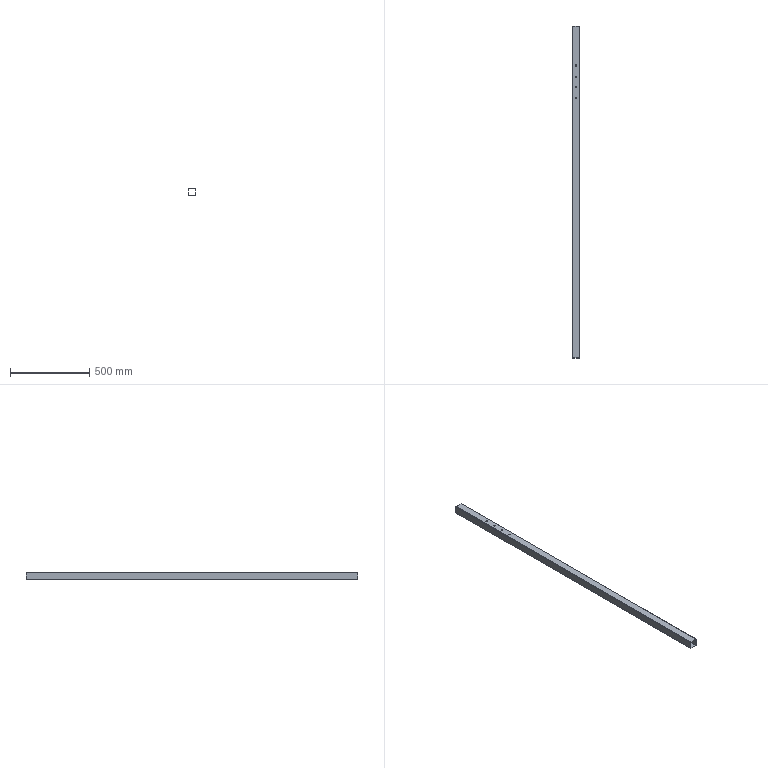Part | SolidWorks | features Extrusion 1, ICE 1 | 1 solid | 34 faces | box 50 x 2097 x 50 mm | volume 900278 mm3 | cylinder 24 | plane 10 | commonest cylinder face diameters 8 x16 2.3 x4 6.9 x4
STEP:
#1=CARTESIAN_POINT('',(4.,1847.,25.));
#2=VERTEX_POINT('',#1);
#3=CARTESIAN_POINT('',(-4.,1847.,25.));
#4=VERTEX_POINT('',#3);
#5=CARTESIAN_POINT('',(0.,1847.,25.));
#6=DIRECTION('',(0.,0.,-1.));
#7=DIRECTION('',(-1.,0.,0.));
#8=AXIS2_PLACEMENT_3D('',#5,#6,#7);
#9=CIRCLE('',#8,4.);
#10=EDGE_CURVE('',#2,#4,#9,.T.);
#11=ORIENTED_EDGE('',*,*,#10,.F.);
#12=CARTESIAN_POINT('',(4.,1847.,22.7));
#13=VERTEX_POINT('',#12);
#14=CARTESIAN_POINT('',(4.,1847.,25.));
#15=DIRECTION('',(0.,0.,-1.));
#16=VECTOR('',#15,1000.);
#17=LINE('',#14,#16);
#18=EDGE_CURVE('',#2,#13,#17,.T.);
#19=ORIENTED_EDGE('',*,*,#18,.T.);
#20=CARTESIAN_POINT('',(-4.,1847.,22.7));
#21=VERTEX_POINT('',#20);
#22=CARTESIAN_POINT('',(0.,1847.,22.7));
#23=DIRECTION('',(0.,0.,-1.));
#24=DIRECTION('',(-1.,0.,0.));
#25=AXIS2_PLACEMENT_3D('',#22,#23,#24);
#26=CIRCLE('',#25,4.);
#27=EDGE_CURVE('',#13,#21,#26,.T.);
#28=ORIENTED_EDGE('',*,*,#27,.T.);
#29=CARTESIAN_POINT('',(-4.,1847.,25.));
#30=DIRECTION('',(0.,0.,-1.));
#31=VECTOR('',#30,1000.);
#32=LINE('',#29,#31);
#33=EDGE_CURVE('',#4,#21,#32,.T.);
#34=ORIENTED_EDGE('',*,*,#33,.F.);
#35=EDGE_LOOP('',(#11,#19,#28,#34));
#36=FACE_OUTER_BOUND('',#35,.T.);
#37=CARTESIAN_POINT('',(0.,1847.,25.));
#38=DIRECTION('',(0.,0.,-1.));
#39=DIRECTION('',(-1.,0.,0.));
#40=AXIS2_PLACEMENT_3D('',#37,#38,#39);
#41=CYLINDRICAL_SURFACE('',#40,4.);
#42=ADVANCED_FACE('',(#36),#41,.F.);
#43=CARTESIAN_POINT('',(4.,1777.,25.));
#44=VERTEX_POINT('',#43);
#45=CARTESIAN_POINT('',(-4.,1777.,25.));
#46=VERTEX_POINT('',#45);
#47=CARTESIAN_POINT('',(0.,1777.,25.));
#48=DIRECTION('',(0.,0.,-1.));
#49=DIRECTION('',(-1.,0.,0.));
#50=AXIS2_PLACEMENT_3D('',#47,#48,#49);
#51=CIRCLE('',#50,4.);
#52=EDGE_CURVE('',#44,#46,#51,.T.);
#53=ORIENTED_EDGE('',*,*,#52,.F.);
#54=CARTESIAN_POINT('',(4.,1777.,22.7));
#55=VERTEX_POINT('',#54);
#56=CARTESIAN_POINT('',(4.,1777.,25.));
#57=DIRECTION('',(0.,0.,-1.));
#58=VECTOR('',#57,1000.);
#59=LINE('',#56,#58);
#60=EDGE_CURVE('',#44,#55,#59,.T.);
#61=ORIENTED_EDGE('',*,*,#60,.T.);
#62=CARTESIAN_POINT('',(-4.,1777.,22.7));
#63=VERTEX_POINT('',#62);
#64=CARTESIAN_POINT('',(0.,1777.,22.7));
#65=DIRECTION('',(0.,0.,-1.));
#66=DIRECTION('',(-1.,0.,0.));
#67=AXIS2_PLACEMENT_3D('',#64,#65,#66);
#68=CIRCLE('',#67,4.);
#69=EDGE_CURVE('',#55,#63,#68,.T.);
#70=ORIENTED_EDGE('',*,*,#69,.T.);
#71=CARTESIAN_POINT('',(-4.,1777.,25.));
#72=DIRECTION('',(0.,0.,-1.));
#73=VECTOR('',#72,1000.);
#74=LINE('',#71,#73);
#75=EDGE_CURVE('',#46,#63,#74,.T.);
#76=ORIENTED_EDGE('',*,*,#75,.F.);
#77=EDGE_LOOP('',(#53,#61,#70,#76));
#78=FACE_OUTER_BOUND('',#77,.T.);
#79=CARTESIAN_POINT('',(0.,1777.,25.));
#80=DIRECTION('',(0.,0.,-1.));
#81=DIRECTION('',(-1.,0.,0.));
#82=AXIS2_PLACEMENT_3D('',#79,#80,#81);
#83=CYLINDRICAL_SURFACE('',#82,4.);
#84=ADVANCED_FACE('',(#78),#83,.F.);
#85=CARTESIAN_POINT('',(4.,1712.,25.));
#86=VERTEX_POINT('',#85);
#87=CARTESIAN_POINT('',(-4.,1712.,25.));
#88=VERTEX_POINT('',#87);
#89=CARTESIAN_POINT('',(0.,1712.,25.));
#90=DIRECTION('',(0.,0.,-1.));
#91=DIRECTION('',(-1.,0.,0.));
#92=AXIS2_PLACEMENT_3D('',#89,#90,#91);
#93=CIRCLE('',#92,4.);
#94=EDGE_CURVE('',#86,#88,#93,.T.);
#95=ORIENTED_EDGE('',*,*,#94,.F.);
#96=CARTESIAN_POINT('',(4.,1712.,22.7));
#97=VERTEX_POINT('',#96);
#98=CARTESIAN_POINT('',(4.,1712.,25.));
#99=DIRECTION('',(0.,0.,-1.));
#100=VECTOR('',#99,1000.);
#101=LINE('',#98,#100);
#102=EDGE_CURVE('',#86,#97,#101,.T.);
#103=ORIENTED_EDGE('',*,*,#102,.T.);
#104=CARTESIAN_POINT('',(-4.,1712.,22.7));
#105=VERTEX_POINT('',#104);
#106=CARTESIAN_POINT('',(0.,1712.,22.7));
#107=DIRECTION('',(0.,0.,-1.));
#108=DIRECTION('',(-1.,0.,0.));
#109=AXIS2_PLACEMENT_3D('',#106,#107,#108);
#110=CIRCLE('',#109,4.);
#111=EDGE_CURVE('',#97,#105,#110,.T.);
#112=ORIENTED_EDGE('',*,*,#111,.T.);
#113=CARTESIAN_POINT('',(-4.,1712.,25.));
#114=DIRECTION('',(0.,0.,-1.));
#115=VECTOR('',#114,1000.);
#116=LINE('',#113,#115);
#117=EDGE_CURVE('',#88,#105,#116,.T.);
#118=ORIENTED_EDGE('',*,*,#117,.F.);
#119=EDGE_LOOP('',(#95,#103,#112,#118));
#120=FACE_OUTER_BOUND('',#119,.T.);
#121=CARTESIAN_POINT('',(0.,1712.,25.));
#122=DIRECTION('',(0.,0.,-1.));
#123=DIRECTION('',(-1.,0.,0.));
#124=AXIS2_PLACEMENT_3D('',#121,#122,#123);
#125=CYLINDRICAL_SURFACE('',#124,4.);
#126=ADVANCED_FACE('',(#120),#125,.F.);
#127=CARTESIAN_POINT('',(4.,1642.,25.));
#128=VERTEX_POINT('',#127);
#129=CARTESIAN_POINT('',(-4.,1642.,25.));
#130=VERTEX_POINT('',#129);
#131=CARTESIAN_POINT('',(0.,1642.,25.));
#132=DIRECTION('',(0.,0.,-1.));
#133=DIRECTION('',(-1.,0.,0.));
#134=AXIS2_PLACEMENT_3D('',#131,#132,#133);
#135=CIRCLE('',#134,4.);
#136=EDGE_CURVE('',#128,#130,#135,.T.);
#137=ORIENTED_EDGE('',*,*,#136,.F.);
#138=CARTESIAN_POINT('',(4.,1642.,22.7));
#139=VERTEX_POINT('',#138);
#140=CARTESIAN_POINT('',(4.,1642.,25.));
#141=DIRECTION('',(0.,0.,-1.));
#142=VECTOR('',#141,1000.);
#143=LINE('',#140,#142);
#144=EDGE_CURVE('',#128,#139,#143,.T.);
#145=ORIENTED_EDGE('',*,*,#144,.T.);
#146=CARTESIAN_POINT('',(-4.,1642.,22.7));
#147=VERTEX_POINT('',#146);
#148=CARTESIAN_POINT('',(0.,1642.,22.7));
#149=DIRECTION('',(0.,0.,-1.));
#150=DIRECTION('',(-1.,0.,0.));
#151=AXIS2_PLACEMENT_3D('',#148,#149,#150);
#152=CIRCLE('',#151,4.);
#153=EDGE_CURVE('',#139,#147,#152,.T.);
#154=ORIENTED_EDGE('',*,*,#153,.T.);
#155=CARTESIAN_POINT('',(-4.,1642.,25.));
#156=DIRECTION('',(0.,0.,-1.));
#157=VECTOR('',#156,1000.);
#158=LINE('',#155,#157);
#159=EDGE_CURVE('',#130,#147,#158,.T.);
#160=ORIENTED_EDGE('',*,*,#159,.F.);
#161=EDGE_LOOP('',(#137,#145,#154,#160));
#162=FACE_OUTER_BOUND('',#161,.T.);
#163=CARTESIAN_POINT('',(0.,1642.,25.));
#164=DIRECTION('',(0.,0.,-1.));
#165=DIRECTION('',(-1.,0.,0.));
#166=AXIS2_PLACEMENT_3D('',#163,#164,#165);
#167=CYLINDRICAL_SURFACE('',#166,4.);
#168=ADVANCED_FACE('',(#162),#167,.F.);
#169=CARTESIAN_POINT('',(-4.,1847.,-22.7));
#170=VERTEX_POINT('',#169);
#171=CARTESIAN_POINT('',(4.,1847.,-22.7));
#172=VERTEX_POINT('',#171);
#173=CARTESIAN_POINT('',(0.,1847.,-22.7));
#174=DIRECTION('',(0.,0.,1.));
#175=DIRECTION('',(1.,0.,0.));
#176=AXIS2_PLACEMENT_3D('',#173,#174,#175);
#177=CIRCLE('',#176,4.);
#178=EDGE_CURVE('',#170,#172,#177,.T.);
#179=ORIENTED_EDGE('',*,*,#178,.T.);
#180=CARTESIAN_POINT('',(4.,1847.,-25.));
#181=VERTEX_POINT('',#180);
#182=CARTESIAN_POINT('',(4.,1847.,25.));
#183=DIRECTION('',(0.,0.,-1.));
#184=VECTOR('',#183,1000.);
#185=LINE('',#182,#184);
#186=EDGE_CURVE('',#172,#181,#185,.T.);
#187=ORIENTED_EDGE('',*,*,#186,.T.);
#188=CARTESIAN_POINT('',(-4.,1847.,-25.));
#189=VERTEX_POINT('',#188);
#190=CARTESIAN_POINT('',(0.,1847.,-25.));
#191=DIRECTION('',(0.,0.,1.));
#192=DIRECTION('',(1.,0.,0.));
#193=AXIS2_PLACEMENT_3D('',#190,#191,#192);
#194=CIRCLE('',#193,4.);
#195=EDGE_CURVE('',#189,#181,#194,.T.);
#196=ORIENTED_EDGE('',*,*,#195,.F.);
#197=CARTESIAN_POINT('',(-4.,1847.,25.));
#198=DIRECTION('',(0.,0.,-1.));
#199=VECTOR('',#198,1000.);
#200=LINE('',#197,#199);
#201=EDGE_CURVE('',#170,#189,#200,.T.);
#202=ORIENTED_EDGE('',*,*,#201,.F.);
#203=EDGE_LOOP('',(#179,#187,#196,#202));
#204=FACE_OUTER_BOUND('',#203,.T.);
#205=CARTESIAN_POINT('',(0.,1847.,25.));
#206=DIRECTION('',(0.,0.,-1.));
#207=DIRECTION('',(-1.,0.,0.));
#208=AXIS2_PLACEMENT_3D('',#205,#206,#207);
#209=CYLINDRICAL_SURFACE('',#208,4.);
#210=ADVANCED_FACE('',(#204),#209,.F.);
#211=CARTESIAN_POINT('',(-4.,1777.,-22.7));
#212=VERTEX_POINT('',#211);
#213=CARTESIAN_POINT('',(4.,1777.,-22.7));
#214=VERTEX_POINT('',#213);
#215=CARTESIAN_POINT('',(0.,1777.,-22.7));
#216=DIRECTION('',(0.,0.,1.));
#217=DIRECTION('',(1.,0.,0.));
#218=AXIS2_PLACEMENT_3D('',#215,#216,#217);
#219=CIRCLE('',#218,4.);
#220=EDGE_CURVE('',#212,#214,#219,.T.);
#221=ORIENTED_EDGE('',*,*,#220,.T.);
#222=CARTESIAN_POINT('',(4.,1777.,-25.));
#223=VERTEX_POINT('',#222);
#224=CARTESIAN_POINT('',(4.,1777.,25.));
#225=DIRECTION('',(0.,0.,-1.));
#226=VECTOR('',#225,1000.);
#227=LINE('',#224,#226);
#228=EDGE_CURVE('',#214,#223,#227,.T.);
#229=ORIENTED_EDGE('',*,*,#228,.T.);
#230=CARTESIAN_POINT('',(-4.,1777.,-25.));
#231=VERTEX_POINT('',#230);
#232=CARTESIAN_POINT('',(0.,1777.,-25.));
#233=DIRECTION('',(0.,0.,1.));
#234=DIRECTION('',(1.,0.,0.));
#235=AXIS2_PLACEMENT_3D('',#232,#233,#234);
#236=CIRCLE('',#235,4.);
#237=EDGE_CURVE('',#231,#223,#236,.T.);
#238=ORIENTED_EDGE('',*,*,#237,.F.);
#239=CARTESIAN_POINT('',(-4.,1777.,25.));
#240=DIRECTION('',(0.,0.,-1.));
#241=VECTOR('',#240,1000.);
#242=LINE('',#239,#241);
#243=EDGE_CURVE('',#212,#231,#242,.T.);
#244=ORIENTED_EDGE('',*,*,#243,.F.);
#245=EDGE_LOOP('',(#221,#229,#238,#244));
#246=FACE_OUTER_BOUND('',#245,.T.);
#247=CARTESIAN_POINT('',(0.,1777.,25.));
#248=DIRECTION('',(0.,0.,-1.));
#249=DIRECTION('',(-1.,0.,0.));
#250=AXIS2_PLACEMENT_3D('',#247,#248,#249);
#251=CYLINDRICAL_SURFACE('',#250,4.);
#252=ADVANCED_FACE('',(#246),#251,.F.);
#253=CARTESIAN_POINT('',(-4.,1712.,-22.7));
#254=VERTEX_POINT('',#253);
#255=CARTESIAN_POINT('',(4.,1712.,-22.7));
#256=VERTEX_POINT('',#255);
#257=CARTESIAN_POINT('',(0.,1712.,-22.7));
#258=DIRECTION('',(0.,0.,1.));
#259=DIRECTION('',(1.,0.,0.));
#260=AXIS2_PLACEMENT_3D('',#257,#258,#259);
#261=CIRCLE('',#260,4.);
#262=EDGE_CURVE('',#254,#256,#261,.T.);
#263=ORIENTED_EDGE('',*,*,#262,.T.);
#264=CARTESIAN_POINT('',(4.,1712.,-25.));
#265=VERTEX_POINT('',#264);
#266=CARTESIAN_POINT('',(4.,1712.,25.));
#267=DIRECTION('',(0.,0.,-1.));
#268=VECTOR('',#267,1000.);
#269=LINE('',#266,#268);
#270=EDGE_CURVE('',#256,#265,#269,.T.);
#271=ORIENTED_EDGE('',*,*,#270,.T.);
#272=CARTESIAN_POINT('',(-4.,1712.,-25.));
#273=VERTEX_POINT('',#272);
#274=CARTESIAN_POINT('',(0.,1712.,-25.));
#275=DIRECTION('',(0.,0.,1.));
#276=DIRECTION('',(1.,0.,0.));
#277=AXIS2_PLACEMENT_3D('',#274,#275,#276);
#278=CIRCLE('',#277,4.);
#279=EDGE_CURVE('',#273,#265,#278,.T.);
#280=ORIENTED_EDGE('',*,*,#279,.F.);
#281=CARTESIAN_POINT('',(-4.,1712.,25.));
#282=DIRECTION('',(0.,0.,-1.));
#283=VECTOR('',#282,1000.);
#284=LINE('',#281,#283);
#285=EDGE_CURVE('',#254,#273,#284,.T.);
#286=ORIENTED_EDGE('',*,*,#285,.F.);
#287=EDGE_LOOP('',(#263,#271,#280,#286));
#288=FACE_OUTER_BOUND('',#287,.T.);
#289=CARTESIAN_POINT('',(0.,1712.,25.));
#290=DIRECTION('',(0.,0.,-1.));
#291=DIRECTION('',(-1.,0.,0.));
#292=AXIS2_PLACEMENT_3D('',#289,#290,#291);
#293=CYLINDRICAL_SURFACE('',#292,4.);
#294=ADVANCED_FACE('',(#288),#293,.F.);
#295=CARTESIAN_POINT('',(-4.,1642.,-22.7));
#296=VERTEX_POINT('',#295);
#297=CARTESIAN_POINT('',(4.,1642.,-22.7));
#298=VERTEX_POINT('',#297);
#299=CARTESIAN_POINT('',(0.,1642.,-22.7));
#300=DIRECTION('',(0.,0.,1.));
#301=DIRECTION('',(1.,0.,0.));
#302=AXIS2_PLACEMENT_3D('',#299,#300,#301);
#303=CIRCLE('',#302,4.);
#304=EDGE_CURVE('',#296,#298,#303,.T.);
#305=ORIENTED_EDGE('',*,*,#304,.T.);
#306=CARTESIAN_POINT('',(4.,1642.,-25.));
#307=VERTEX_POINT('',#306);
#308=CARTESIAN_POINT('',(4.,1642.,25.));
#309=DIRECTION('',(0.,0.,-1.));
#310=VECTOR('',#309,1000.);
#311=LINE('',#308,#310);
#312=EDGE_CURVE('',#298,#307,#311,.T.);
#313=ORIENTED_EDGE('',*,*,#312,.T.);
#314=CARTESIAN_POINT('',(-4.,1642.,-25.));
#315=VERTEX_POINT('',#314);
#316=CARTESIAN_POINT('',(0.,1642.,-25.));
#317=DIRECTION('',(0.,0.,1.));
#318=DIRECTION('',(1.,0.,0.));
#319=AXIS2_PLACEMENT_3D('',#316,#317,#318);
#320=CIRCLE('',#319,4.);
#321=EDGE_CURVE('',#315,#307,#320,.T.);
#322=ORIENTED_EDGE('',*,*,#321,.F.);
#323=CARTESIAN_POINT('',(-4.,1642.,25.));
#324=DIRECTION('',(0.,0.,-1.));
#325=VECTOR('',#324,1000.);
#326=LINE('',#323,#325);
#327=EDGE_CURVE('',#296,#315,#326,.T.);
#328=ORIENTED_EDGE('',*,*,#327,.F.);
#329=EDGE_LOOP('',(#305,#313,#322,#328));
#330=FACE_OUTER_BOUND('',#329,.T.);
#331=CARTESIAN_POINT('',(0.,1642.,25.));
#332=DIRECTION('',(0.,0.,-1.));
#333=DIRECTION('',(-1.,0.,0.));
#334=AXIS2_PLACEMENT_3D('',#331,#332,#333);
#335=CYLINDRICAL_SURFACE('',#334,4.);
#336=ADVANCED_FACE('',(#330),#335,.F.);
#337=CARTESIAN_POINT('',(25.,2097.,-21.55));
#338=VERTEX_POINT('',#337);
#339=CARTESIAN_POINT('',(21.55,2097.,-25.));
#340=VERTEX_POINT('',#339);
#341=CARTESIAN_POINT('',(21.55,2097.,-21.55));
#342=DIRECTION('',(0.,1.,0.));
#343=DIRECTION('',(0.,0.,-1.));
#344=AXIS2_PLACEMENT_3D('',#341,#342,#343);
#345=CIRCLE('',#344,3.45);
#346=EDGE_CURVE('',#338,#340,#345,.T.);
#347=ORIENTED_EDGE('',*,*,#346,.T.);
#348=CARTESIAN_POINT('',(-21.55,2097.,-25.));
#349=VERTEX_POINT('',#348);
#350=CARTESIAN_POINT('',(-21.55,2097.,-25.));
#351=DIRECTION('',(-1.,0.,0.));
#352=VECTOR('',#351,1000.);
#353=LINE('',#350,#352);
#354=EDGE_CURVE('',#340,#349,#353,.T.);
#355=ORIENTED_EDGE('',*,*,#354,.T.);
#356=CARTESIAN_POINT('',(-25.,2097.,-21.55));
#357=VERTEX_POINT('',#356);
#358=CARTESIAN_POINT('',(-21.55,2097.,-21.55));
#359=DIRECTION('',(0.,1.,0.));
#360=DIRECTION('',(0.,0.,-1.));
#361=AXIS2_PLACEMENT_3D('',#358,#359,#360);
#362=CIRCLE('',#361,3.45);
#363=EDGE_CURVE('',#349,#357,#362,.T.);
#364=ORIENTED_EDGE('',*,*,#363,.T.);
#365=CARTESIAN_POINT('',(-25.,2097.,21.55));
#366=VERTEX_POINT('',#365);
#367=CARTESIAN_POINT('',(-25.,2097.,21.55));
#368=DIRECTION('',(0.,0.,1.));
#369=VECTOR('',#368,1000.);
#370=LINE('',#367,#369);
#371=EDGE_CURVE('',#357,#366,#370,.T.);
#372=ORIENTED_EDGE('',*,*,#371,.T.);
#373=CARTESIAN_POINT('',(-21.55,2097.,25.));
#374=VERTEX_POINT('',#373);
#375=CARTESIAN_POINT('',(-21.55,2097.,21.55));
#376=DIRECTION('',(0.,1.,0.));
#377=DIRECTION('',(0.,0.,-1.));
#378=AXIS2_PLACEMENT_3D('',#375,#376,#377);
#379=CIRCLE('',#378,3.45);
#380=EDGE_CURVE('',#366,#374,#379,.T.);
#381=ORIENTED_EDGE('',*,*,#380,.T.);
#382=CARTESIAN_POINT('',(21.55,2097.,25.));
#383=VERTEX_POINT('',#382);
#384=CARTESIAN_POINT('',(-21.55,2097.,25.));
#385=DIRECTION('',(1.,0.,0.));
#386=VECTOR('',#385,1000.);
#387=LINE('',#384,#386);
#388=EDGE_CURVE('',#374,#383,#387,.T.);
#389=ORIENTED_EDGE('',*,*,#388,.T.);
#390=CARTESIAN_POINT('',(25.,2097.,21.55));
#391=VERTEX_POINT('',#390);
#392=CARTESIAN_POINT('',(21.55,2097.,21.55));
#393=DIRECTION('',(0.,1.,0.));
#394=DIRECTION('',(0.,0.,1.));
#395=AXIS2_PLACEMENT_3D('',#392,#393,#394);
#396=CIRCLE('',#395,3.45);
#397=EDGE_CURVE('',#383,#391,#396,.T.);
#398=ORIENTED_EDGE('',*,*,#397,.T.);
#399=CARTESIAN_POINT('',(25.,2097.,21.55));
#400=DIRECTION('',(0.,0.,-1.));
#401=VECTOR('',#400,1000.);
#402=LINE('',#399,#401);
#403=EDGE_CURVE('',#391,#338,#402,.T.);
#404=ORIENTED_EDGE('',*,*,#403,.T.);
#405=EDGE_LOOP('',(#347,#355,#364,#372,#381,#389,#398,#404));
#406=FACE_OUTER_BOUND('',#405,.T.);
#407=CARTESIAN_POINT('',(-22.7,2097.,21.55));
#408=VERTEX_POINT('',#407);
#409=CARTESIAN_POINT('',(-21.55,2097.,22.7));
#410=VERTEX_POINT('',#409);
#411=CARTESIAN_POINT('',(-21.55,2097.,21.55));
#412=DIRECTION('',(0.,1.,0.));
#413=DIRECTION('',(0.,0.,-1.));
#414=AXIS2_PLACEMENT_3D('',#411,#412,#413);
#415=CIRCLE('',#414,1.15);
#416=EDGE_CURVE('',#408,#410,#415,.T.);
#417=ORIENTED_EDGE('',*,*,#416,.F.);
#418=CARTESIAN_POINT('',(-22.7,2097.,-21.55));
#419=VERTEX_POINT('',#418);
#420=CARTESIAN_POINT('',(-22.7,2097.,21.55));
#421=DIRECTION('',(0.,0.,1.));
#422=VECTOR('',#421,1000.);
#423=LINE('',#420,#422);
#424=EDGE_CURVE('',#419,#408,#423,.T.);
#425=ORIENTED_EDGE('',*,*,#424,.F.);
#426=CARTESIAN_POINT('',(-21.55,2097.,-22.7));
#427=VERTEX_POINT('',#426);
#428=CARTESIAN_POINT('',(-21.55,2097.,-21.55));
#429=DIRECTION('',(0.,1.,0.));
#430=DIRECTION('',(0.,0.,-1.));
#431=AXIS2_PLACEMENT_3D('',#428,#429,#430);
#432=CIRCLE('',#431,1.15);
#433=EDGE_CURVE('',#427,#419,#432,.T.);
#434=ORIENTED_EDGE('',*,*,#433,.F.);
#435=CARTESIAN_POINT('',(21.55,2097.,-22.7));
#436=VERTEX_POINT('',#435);
#437=CARTESIAN_POINT('',(-21.55,2097.,-22.7));
#438=DIRECTION('',(-1.,0.,0.));
#439=VECTOR('',#438,1000.);
#440=LINE('',#437,#439);
#441=EDGE_CURVE('',#436,#427,#440,.T.);
#442=ORIENTED_EDGE('',*,*,#441,.F.);
#443=CARTESIAN_POINT('',(22.7,2097.,-21.55));
#444=VERTEX_POINT('',#443);
#445=CARTESIAN_POINT('',(21.55,2097.,-21.55));
#446=DIRECTION('',(0.,1.,0.));
#447=DIRECTION('',(0.,0.,-1.));
#448=AXIS2_PLACEMENT_3D('',#445,#446,#447);
#449=CIRCLE('',#448,1.15);
#450=EDGE_CURVE('',#444,#436,#449,.T.);
#451=ORIENTED_EDGE('',*,*,#450,.F.);
#452=CARTESIAN_POINT('',(22.7,2097.,21.55));
#453=VERTEX_POINT('',#452);
#454=CARTESIAN_POINT('',(22.7,2097.,21.55));
#455=DIRECTION('',(0.,0.,-1.));
#456=VECTOR('',#455,1000.);
#457=LINE('',#454,#456);
#458=EDGE_CURVE('',#453,#444,#457,.T.);
#459=ORIENTED_EDGE('',*,*,#458,.F.);
#460=CARTESIAN_POINT('',(21.55,2097.,22.7));
#461=VERTEX_POINT('',#460);
#462=CARTESIAN_POINT('',(21.55,2097.,21.55));
#463=DIRECTION('',(0.,1.,0.));
#464=DIRECTION('',(0.,0.,1.));
#465=AXIS2_PLACEMENT_3D('',#462,#463,#464);
#466=CIRCLE('',#465,1.15);
#467=EDGE_CURVE('',#461,#453,#466,.T.);
#468=ORIENTED_EDGE('',*,*,#467,.F.);
#469=CARTESIAN_POINT('',(-21.55,2097.,22.7));
#470=DIRECTION('',(1.,0.,0.));
#471=VECTOR('',#470,1000.);
#472=LINE('',#469,#471);
#473=EDGE_CURVE('',#410,#461,#472,.T.);
#474=ORIENTED_EDGE('',*,*,#473,.F.);
#475=EDGE_LOOP('',(#417,#425,#434,#442,#451,#459,#468,#474));
#476=FACE_BOUND('',#475,.T.);
#477=CARTESIAN_POINT('',(21.55,2097.,-21.55));
#478=DIRECTION('',(0.,-1.,0.));
#479=DIRECTION('',(0.,0.,-1.));
#480=AXIS2_PLACEMENT_3D('',#477,#478,#479);
#481=PLANE('',#480);
#482=ADVANCED_FACE('',(#406,#476),#481,.F.);
#483=CARTESIAN_POINT('',(25.,0.,-21.55));
#484=VERTEX_POINT('',#483);
#485=CARTESIAN_POINT('',(21.55,0.,-25.));
#486=VERTEX_POINT('',#485);
#487=CARTESIAN_POINT('',(21.55,0.,-21.55));
#488=DIRECTION('',(0.,1.,0.));
#489=DIRECTION('',(0.,0.,-1.));
#490=AXIS2_PLACEMENT_3D('',#487,#488,#489);
#491=CIRCLE('',#490,3.45);
#492=EDGE_CURVE('',#484,#486,#491,.T.);
#493=ORIENTED_EDGE('',*,*,#492,.F.);
#494=CARTESIAN_POINT('',(25.,0.,21.55));
#495=VERTEX_POINT('',#494);
#496=CARTESIAN_POINT('',(25.,0.,21.55));
#497=DIRECTION('',(0.,0.,-1.));
#498=VECTOR('',#497,1000.);
#499=LINE('',#496,#498);
#500=EDGE_CURVE('',#495,#484,#499,.T.);
#501=ORIENTED_EDGE('',*,*,#500,.F.);
#502=CARTESIAN_POINT('',(21.55,0.,25.));
#503=VERTEX_POINT('',#502);
#504=CARTESIAN_POINT('',(21.55,0.,21.55));
#505=DIRECTION('',(0.,1.,0.));
#506=DIRECTION('',(0.,0.,1.));
#507=AXIS2_PLACEMENT_3D('',#504,#505,#506);
#508=CIRCLE('',#507,3.45);
#509=EDGE_CURVE('',#503,#495,#508,.T.);
#510=ORIENTED_EDGE('',*,*,#509,.F.);
#511=CARTESIAN_POINT('',(-21.55,0.,25.));
#512=VERTEX_POINT('',#511);
#513=CARTESIAN_POINT('',(-21.55,0.,25.));
#514=DIRECTION('',(1.,0.,0.));
#515=VECTOR('',#514,1000.);
#516=LINE('',#513,#515);
#517=EDGE_CURVE('',#512,#503,#516,.T.);
#518=ORIENTED_EDGE('',*,*,#517,.F.);
#519=CARTESIAN_POINT('',(-25.,0.,21.55));
#520=VERTEX_POINT('',#519);
#521=CARTESIAN_POINT('',(-21.55,0.,21.55));
#522=DIRECTION('',(0.,1.,0.));
#523=DIRECTION('',(0.,0.,-1.));
#524=AXIS2_PLACEMENT_3D('',#521,#522,#523);
#525=CIRCLE('',#524,3.45);
#526=EDGE_CURVE('',#520,#512,#525,.T.);
#527=ORIENTED_EDGE('',*,*,#526,.F.);
#528=CARTESIAN_POINT('',(-25.,0.,-21.55));
#529=VERTEX_POINT('',#528);
#530=CARTESIAN_POINT('',(-25.,0.,21.55));
#531=DIRECTION('',(0.,0.,1.));
#532=VECTOR('',#531,1000.);
#533=LINE('',#530,#532);
#534=EDGE_CURVE('',#529,#520,#533,.T.);
#535=ORIENTED_EDGE('',*,*,#534,.F.);
#536=CARTESIAN_POINT('',(-21.55,0.,-25.));
#537=VERTEX_POINT('',#536);
#538=CARTESIAN_POINT('',(-21.55,0.,-21.55));
#539=DIRECTION('',(0.,1.,0.));
#540=DIRECTION('',(0.,0.,-1.));
#541=AXIS2_PLACEMENT_3D('',#538,#539,#540);
#542=CIRCLE('',#541,3.45);
#543=EDGE_CURVE('',#537,#529,#542,.T.);
#544=ORIENTED_EDGE('',*,*,#543,.F.);
#545=CARTESIAN_POINT('',(-21.55,0.,-25.));
#546=DIRECTION('',(-1.,0.,0.));
#547=VECTOR('',#546,1000.);
#548=LINE('',#545,#547);
#549=EDGE_CURVE('',#486,#537,#548,.T.);
#550=ORIENTED_EDGE('',*,*,#549,.F.);
#551=EDGE_LOOP('',(#493,#501,#510,#518,#527,#535,#544,#550));
#552=FACE_OUTER_BOUND('',#551,.T.);
#553=CARTESIAN_POINT('',(-22.7,0.,-21.55));
#554=VERTEX_POINT('',#553);
#555=CARTESIAN_POINT('',(-22.7,0.,21.55));
#556=VERTEX_POINT('',#555);
#557=CARTESIAN_POINT('',(-22.7,0.,21.55));
#558=DIRECTION('',(0.,0.,1.));
#559=VECTOR('',#558,1000.);
#560=LINE('',#557,#559);
#561=EDGE_CURVE('',#554,#556,#560,.T.);
#562=ORIENTED_EDGE('',*,*,#561,.T.);
#563=CARTESIAN_POINT('',(-21.55,0.,22.7));
#564=VERTEX_POINT('',#563);
#565=CARTESIAN_POINT('',(-21.55,0.,21.55));
#566=DIRECTION('',(0.,1.,0.));
#567=DIRECTION('',(0.,0.,-1.));
#568=AXIS2_PLACEMENT_3D('',#565,#566,#567);
#569=CIRCLE('',#568,1.15);
#570=EDGE_CURVE('',#556,#564,#569,.T.);
#571=ORIENTED_EDGE('',*,*,#570,.T.);
#572=CARTESIAN_POINT('',(21.55,0.,22.7));
#573=VERTEX_POINT('',#572);
#574=CARTESIAN_POINT('',(-21.55,0.,22.7));
#575=DIRECTION('',(1.,0.,0.));
#576=VECTOR('',#575,1000.);
#577=LINE('',#574,#576);
#578=EDGE_CURVE('',#564,#573,#577,.T.);
#579=ORIENTED_EDGE('',*,*,#578,.T.);
#580=CARTESIAN_POINT('',(22.7,0.,21.55));
#581=VERTEX_POINT('',#580);
#582=CARTESIAN_POINT('',(21.55,0.,21.55));
#583=DIRECTION('',(0.,1.,0.));
#584=DIRECTION('',(0.,0.,1.));
#585=AXIS2_PLACEMENT_3D('',#582,#583,#584);
#586=CIRCLE('',#585,1.15);
#587=EDGE_CURVE('',#573,#581,#586,.T.);
#588=ORIENTED_EDGE('',*,*,#587,.T.);
#589=CARTESIAN_POINT('',(22.7,0.,-21.55));
#590=VERTEX_POINT('',#589);
#591=CARTESIAN_POINT('',(22.7,0.,21.55));
#592=DIRECTION('',(0.,0.,-1.));
#593=VECTOR('',#592,1000.);
#594=LINE('',#591,#593);
#595=EDGE_CURVE('',#581,#590,#594,.T.);
#596=ORIENTED_EDGE('',*,*,#595,.T.);
#597=CARTESIAN_POINT('',(21.55,0.,-22.7));
#598=VERTEX_POINT('',#597);
#599=CARTESIAN_POINT('',(21.55,0.,-21.55));
#600=DIRECTION('',(0.,1.,0.));
#601=DIRECTION('',(0.,0.,-1.));
#602=AXIS2_PLACEMENT_3D('',#599,#600,#601);
#603=CIRCLE('',#602,1.15);
#604=EDGE_CURVE('',#590,#598,#603,.T.);
#605=ORIENTED_EDGE('',*,*,#604,.T.);
#606=CARTESIAN_POINT('',(-21.55,0.,-22.7));
#607=VERTEX_POINT('',#606);
#608=CARTESIAN_POINT('',(-21.55,0.,-22.7));
#609=DIRECTION('',(-1.,0.,0.));
#610=VECTOR('',#609,1000.);
#611=LINE('',#608,#610);
#612=EDGE_CURVE('',#598,#607,#611,.T.);
#613=ORIENTED_EDGE('',*,*,#612,.T.);
#614=CARTESIAN_POINT('',(-21.55,0.,-21.55));
#615=DIRECTION('',(0.,1.,0.));
#616=DIRECTION('',(0.,0.,-1.));
#617=AXIS2_PLACEMENT_3D('',#614,#615,#616);
#618=CIRCLE('',#617,1.15);
#619=EDGE_CURVE('',#607,#554,#618,.T.);
#620=ORIENTED_EDGE('',*,*,#619,.T.);
#621=EDGE_LOOP('',(#562,#571,#579,#588,#596,#605,#613,#620));
#622=FACE_BOUND('',#621,.T.);
#623=CARTESIAN_POINT('',(21.55,0.,-21.55));
#624=DIRECTION('',(0.,-1.,0.));
#625=DIRECTION('',(0.,0.,-1.));
#626=AXIS2_PLACEMENT_3D('',#623,#624,#625);
#627=PLANE('',#626);
#628=ADVANCED_FACE('',(#552,#622),#627,.T.);
#629=ORIENTED_EDGE('',*,*,#492,.T.);
#630=CARTESIAN_POINT('',(21.55,2097.,-25.));
#631=DIRECTION('',(0.,-1.,0.));
#632=VECTOR('',#631,1000.);
#633=LINE('',#630,#632);
#634=EDGE_CURVE('',#340,#486,#633,.T.);
#635=ORIENTED_EDGE('',*,*,#634,.F.);
#636=ORIENTED_EDGE('',*,*,#346,.F.);
#637=CARTESIAN_POINT('',(25.,2097.,-21.55));
#638=DIRECTION('',(0.,-1.,0.));
#639=VECTOR('',#638,1000.);
#640=LINE('',#637,#639);
#641=EDGE_CURVE('',#338,#484,#640,.T.);
#642=ORIENTED_EDGE('',*,*,#641,.T.);
#643=EDGE_LOOP('',(#629,#635,#636,#642));
#644=FACE_OUTER_BOUND('',#643,.T.);
#645=CARTESIAN_POINT('',(21.55,2097.,-21.55));
#646=DIRECTION('',(0.,-1.,0.));
#647=DIRECTION('',(0.,0.,-1.));
#648=AXIS2_PLACEMENT_3D('',#645,#646,#647);
#649=CYLINDRICAL_SURFACE('',#648,3.45);
#650=ADVANCED_FACE('',(#644),#649,.T.);
#651=ORIENTED_EDGE('',*,*,#195,.T.);
#652=CARTESIAN_POINT('',(0.,1847.,-25.));
#653=DIRECTION('',(0.,0.,1.));
#654=DIRECTION('',(1.,0.,0.));
#655=AXIS2_PLACEMENT_3D('',#652,#653,#654);
#656=CIRCLE('',#655,4.);
#657=EDGE_CURVE('',#181,#189,#656,.T.);
#658=ORIENTED_EDGE('',*,*,#657,.T.);
#659=EDGE_LOOP('',(#651,#658));
#660=FACE_BOUND('',#659,.T.);
#661=ORIENTED_EDGE('',*,*,#237,.T.);
#662=CARTESIAN_POINT('',(0.,1777.,-25.));
#663=DIRECTION('',(0.,0.,1.));
#664=DIRECTION('',(1.,0.,0.));
#665=AXIS2_PLACEMENT_3D('',#662,#663,#664);
#666=CIRCLE('',#665,4.);
#667=EDGE_CURVE('',#223,#231,#666,.T.);
#668=ORIENTED_EDGE('',*,*,#667,.T.);
#669=EDGE_LOOP('',(#661,#668));
#670=FACE_BOUND('',#669,.T.);
#671=ORIENTED_EDGE('',*,*,#279,.T.);
#672=CARTESIAN_POINT('',(0.,1712.,-25.));
#673=DIRECTION('',(0.,0.,1.));
#674=DIRECTION('',(1.,0.,0.));
#675=AXIS2_PLACEMENT_3D('',#672,#673,#674);
#676=CIRCLE('',#675,4.);
#677=EDGE_CURVE('',#265,#273,#676,.T.);
#678=ORIENTED_EDGE('',*,*,#677,.T.);
#679=EDGE_LOOP('',(#671,#678));
#680=FACE_BOUND('',#679,.T.);
#681=ORIENTED_EDGE('',*,*,#321,.T.);
#682=CARTESIAN_POINT('',(0.,1642.,-25.));
#683=DIRECTION('',(0.,0.,1.));
#684=DIRECTION('',(1.,0.,0.));
#685=AXIS2_PLACEMENT_3D('',#682,#683,#684);
#686=CIRCLE('',#685,4.);
#687=EDGE_CURVE('',#307,#315,#686,.T.);
#688=ORIENTED_EDGE('',*,*,#687,.T.);
#689=EDGE_LOOP('',(#681,#688));
#690=FACE_BOUND('',#689,.T.);
#691=ORIENTED_EDGE('',*,*,#549,.T.);
#692=CARTESIAN_POINT('',(-21.55,2097.,-25.));
#693=DIRECTION('',(0.,-1.,0.));
#694=VECTOR('',#693,1000.);
#695=LINE('',#692,#694);
#696=EDGE_CURVE('',#349,#537,#695,.T.);
#697=ORIENTED_EDGE('',*,*,#696,.F.);
#698=ORIENTED_EDGE('',*,*,#354,.F.);
#699=ORIENTED_EDGE('',*,*,#634,.T.);
#700=EDGE_LOOP('',(#691,#697,#698,#699));
#701=FACE_OUTER_BOUND('',#700,.T.);
#702=CARTESIAN_POINT('',(-21.55,2097.,-25.));
#703=DIRECTION('',(0.,0.,1.));
#704=DIRECTION('',(1.,0.,0.));
#705=AXIS2_PLACEMENT_3D('',#702,#703,#704);
#706=PLANE('',#705);
#707=ADVANCED_FACE('',(#660,#670,#680,#690,#701),#706,.F.);
#708=ORIENTED_EDGE('',*,*,#543,.T.);
#709=CARTESIAN_POINT('',(-25.,2097.,-21.55));
#710=DIRECTION('',(0.,-1.,0.));
#711=VECTOR('',#710,1000.);
#712=LINE('',#709,#711);
#713=EDGE_CURVE('',#357,#529,#712,.T.);
#714=ORIENTED_EDGE('',*,*,#713,.F.);
#715=ORIENTED_EDGE('',*,*,#363,.F.);
#716=ORIENTED_EDGE('',*,*,#696,.T.);
#717=EDGE_LOOP('',(#708,#714,#715,#716));
#718=FACE_OUTER_BOUND('',#717,.T.);
#719=CARTESIAN_POINT('',(-21.55,2097.,-21.55));
#720=DIRECTION('',(0.,-1.,0.));
#721=DIRECTION('',(0.,0.,-1.));
#722=AXIS2_PLACEMENT_3D('',#719,#720,#721);
#723=CYLINDRICAL_SURFACE('',#722,3.45);
#724=ADVANCED_FACE('',(#718),#723,.T.);
#725=ORIENTED_EDGE('',*,*,#534,.T.);
#726=CARTESIAN_POINT('',(-25.,2097.,21.55));
#727=DIRECTION('',(0.,-1.,0.));
#728=VECTOR('',#727,1000.);
#729=LINE('',#726,#728);
#730=EDGE_CURVE('',#366,#520,#729,.T.);
#731=ORIENTED_EDGE('',*,*,#730,.F.);
#732=ORIENTED_EDGE('',*,*,#371,.F.);
#733=ORIENTED_EDGE('',*,*,#713,.T.);
#734=EDGE_LOOP('',(#725,#731,#732,#733));
#735=FACE_OUTER_BOUND('',#734,.T.);
#736=CARTESIAN_POINT('',(-25.,2097.,21.55));
#737=DIRECTION('',(1.,0.,0.));
#738=DIRECTION('',(0.,0.,-1.));
#739=AXIS2_PLACEMENT_3D('',#736,#737,#738);
#740=PLANE('',#739);
#741=ADVANCED_FACE('',(#735),#740,.F.);
#742=ORIENTED_EDGE('',*,*,#526,.T.);
#743=CARTESIAN_POINT('',(-21.55,2097.,25.));
#744=DIRECTION('',(0.,-1.,0.));
#745=VECTOR('',#744,1000.);
#746=LINE('',#743,#745);
#747=EDGE_CURVE('',#374,#512,#746,.T.);
#748=ORIENTED_EDGE('',*,*,#747,.F.);
#749=ORIENTED_EDGE('',*,*,#380,.F.);
#750=ORIENTED_EDGE('',*,*,#730,.T.);
#751=EDGE_LOOP('',(#742,#748,#749,#750));
#752=FACE_OUTER_BOUND('',#751,.T.);
#753=CARTESIAN_POINT('',(-21.55,2097.,21.55));
#754=DIRECTION('',(0.,-1.,0.));
#755=DIRECTION('',(0.,0.,-1.));
#756=AXIS2_PLACEMENT_3D('',#753,#754,#755);
#757=CYLINDRICAL_SURFACE('',#756,3.45);
#758=ADVANCED_FACE('',(#752),#757,.T.);
#759=CARTESIAN_POINT('',(0.,1847.,25.));
#760=DIRECTION('',(0.,0.,-1.));
#761=DIRECTION('',(-1.,0.,0.));
#762=AXIS2_PLACEMENT_3D('',#759,#760,#761);
#763=CIRCLE('',#762,4.);
#764=EDGE_CURVE('',#4,#2,#763,.T.);
#765=ORIENTED_EDGE('',*,*,#764,.T.);
#766=ORIENTED_EDGE('',*,*,#10,.T.);
#767=EDGE_LOOP('',(#765,#766));
#768=FACE_BOUND('',#767,.T.);
#769=CARTESIAN_POINT('',(0.,1777.,25.));
#770=DIRECTION('',(0.,0.,-1.));
#771=DIRECTION('',(-1.,0.,0.));
#772=AXIS2_PLACEMENT_3D('',#769,#770,#771);
#773=CIRCLE('',#772,4.);
#774=EDGE_CURVE('',#46,#44,#773,.T.);
#775=ORIENTED_EDGE('',*,*,#774,.T.);
#776=ORIENTED_EDGE('',*,*,#52,.T.);
#777=EDGE_LOOP('',(#775,#776));
#778=FACE_BOUND('',#777,.T.);
#779=CARTESIAN_POINT('',(0.,1712.,25.));
#780=DIRECTION('',(0.,0.,-1.));
#781=DIRECTION('',(-1.,0.,0.));
#782=AXIS2_PLACEMENT_3D('',#779,#780,#781);
#783=CIRCLE('',#782,4.);
#784=EDGE_CURVE('',#88,#86,#783,.T.);
#785=ORIENTED_EDGE('',*,*,#784,.T.);
#786=ORIENTED_EDGE('',*,*,#94,.T.);
#787=EDGE_LOOP('',(#785,#786));
#788=FACE_BOUND('',#787,.T.);
#789=CARTESIAN_POINT('',(0.,1642.,25.));
#790=DIRECTION('',(0.,0.,-1.));
#791=DIRECTION('',(-1.,0.,0.));
#792=AXIS2_PLACEMENT_3D('',#789,#790,#791);
#793=CIRCLE('',#792,4.);
#794=EDGE_CURVE('',#130,#128,#793,.T.);
#795=ORIENTED_EDGE('',*,*,#794,.T.);
#796=ORIENTED_EDGE('',*,*,#136,.T.);
#797=EDGE_LOOP('',(#795,#796));
#798=FACE_BOUND('',#797,.T.);
#799=ORIENTED_EDGE('',*,*,#517,.T.);
#800=CARTESIAN_POINT('',(21.55,2097.,25.));
#801=DIRECTION('',(0.,-1.,0.));
#802=VECTOR('',#801,1000.);
#803=LINE('',#800,#802);
#804=EDGE_CURVE('',#383,#503,#803,.T.);
#805=ORIENTED_EDGE('',*,*,#804,.F.);
#806=ORIENTED_EDGE('',*,*,#388,.F.);
#807=ORIENTED_EDGE('',*,*,#747,.T.);
#808=EDGE_LOOP('',(#799,#805,#806,#807));
#809=FACE_OUTER_BOUND('',#808,.T.);
#810=CARTESIAN_POINT('',(-21.55,2097.,25.));
#811=DIRECTION('',(0.,0.,-1.));
#812=DIRECTION('',(-1.,0.,0.));
#813=AXIS2_PLACEMENT_3D('',#810,#811,#812);
#814=PLANE('',#813);
#815=ADVANCED_FACE('',(#768,#778,#788,#798,#809),#814,.F.);
#816=ORIENTED_EDGE('',*,*,#509,.T.);
#817=CARTESIAN_POINT('',(25.,2097.,21.55));
#818=DIRECTION('',(0.,-1.,0.));
#819=VECTOR('',#818,1000.);
#820=LINE('',#817,#819);
#821=EDGE_CURVE('',#391,#495,#820,.T.);
#822=ORIENTED_EDGE('',*,*,#821,.F.);
#823=ORIENTED_EDGE('',*,*,#397,.F.);
#824=ORIENTED_EDGE('',*,*,#804,.T.);
#825=EDGE_LOOP('',(#816,#822,#823,#824));
#826=FACE_OUTER_BOUND('',#825,.T.);
#827=CARTESIAN_POINT('',(21.55,2097.,21.55));
#828=DIRECTION('',(0.,-1.,0.));
#829=DIRECTION('',(0.,0.,-1.));
#830=AXIS2_PLACEMENT_3D('',#827,#828,#829);
#831=CYLINDRICAL_SURFACE('',#830,3.45);
#832=ADVANCED_FACE('',(#826),#831,.T.);
#833=ORIENTED_EDGE('',*,*,#500,.T.);
#834=ORIENTED_EDGE('',*,*,#641,.F.);
#835=ORIENTED_EDGE('',*,*,#403,.F.);
#836=ORIENTED_EDGE('',*,*,#821,.T.);
#837=EDGE_LOOP('',(#833,#834,#835,#836));
#838=FACE_OUTER_BOUND('',#837,.T.);
#839=CARTESIAN_POINT('',(25.,2097.,21.55));
#840=DIRECTION('',(-1.,0.,0.));
#841=DIRECTION('',(0.,0.,1.));
#842=AXIS2_PLACEMENT_3D('',#839,#840,#841);
#843=PLANE('',#842);
#844=ADVANCED_FACE('',(#838),#843,.F.);
#845=ORIENTED_EDGE('',*,*,#570,.F.);
#846=CARTESIAN_POINT('',(-22.7,2097.,21.55));
#847=DIRECTION('',(0.,-1.,0.));
#848=VECTOR('',#847,1000.);
#849=LINE('',#846,#848);
#850=EDGE_CURVE('',#408,#556,#849,.T.);
#851=ORIENTED_EDGE('',*,*,#850,.F.);
#852=ORIENTED_EDGE('',*,*,#416,.T.);
#853=CARTESIAN_POINT('',(-21.55,2097.,22.7));
#854=DIRECTION('',(0.,-1.,0.));
#855=VECTOR('',#854,1000.);
#856=LINE('',#853,#855);
#857=EDGE_CURVE('',#410,#564,#856,.T.);
#858=ORIENTED_EDGE('',*,*,#857,.T.);
#859=EDGE_LOOP('',(#845,#851,#852,#858));
#860=FACE_OUTER_BOUND('',#859,.T.);
#861=CARTESIAN_POINT('',(-21.55,2097.,21.55));
#862=DIRECTION('',(0.,-1.,0.));
#863=DIRECTION('',(0.,0.,-1.));
#864=AXIS2_PLACEMENT_3D('',#861,#862,#863);
#865=CYLINDRICAL_SURFACE('',#864,1.15);
#866=ADVANCED_FACE('',(#860),#865,.F.);
#867=CARTESIAN_POINT('',(0.,1847.,22.7));
#868=DIRECTION('',(0.,0.,-1.));
#869=DIRECTION('',(-1.,0.,0.));
#870=AXIS2_PLACEMENT_3D('',#867,#868,#869);
#871=CIRCLE('',#870,4.);
#872=EDGE_CURVE('',#21,#13,#871,.T.);
#873=ORIENTED_EDGE('',*,*,#872,.F.);
#874=ORIENTED_EDGE('',*,*,#27,.F.);
#875=EDGE_LOOP('',(#873,#874));
#876=FACE_BOUND('',#875,.T.);
#877=CARTESIAN_POINT('',(0.,1777.,22.7));
#878=DIRECTION('',(0.,0.,-1.));
#879=DIRECTION('',(-1.,0.,0.));
#880=AXIS2_PLACEMENT_3D('',#877,#878,#879);
#881=CIRCLE('',#880,4.);
#882=EDGE_CURVE('',#63,#55,#881,.T.);
#883=ORIENTED_EDGE('',*,*,#882,.F.);
#884=ORIENTED_EDGE('',*,*,#69,.F.);
#885=EDGE_LOOP('',(#883,#884));
#886=FACE_BOUND('',#885,.T.);
#887=CARTESIAN_POINT('',(0.,1712.,22.7));
#888=DIRECTION('',(0.,0.,-1.));
#889=DIRECTION('',(-1.,0.,0.));
#890=AXIS2_PLACEMENT_3D('',#887,#888,#889);
#891=CIRCLE('',#890,4.);
#892=EDGE_CURVE('',#105,#97,#891,.T.);
#893=ORIENTED_EDGE('',*,*,#892,.F.);
#894=ORIENTED_EDGE('',*,*,#111,.F.);
#895=EDGE_LOOP('',(#893,#894));
#896=FACE_BOUND('',#895,.T.);
#897=CARTESIAN_POINT('',(0.,1642.,22.7));
#898=DIRECTION('',(0.,0.,-1.));
#899=DIRECTION('',(-1.,0.,0.));
#900=AXIS2_PLACEMENT_3D('',#897,#898,#899);
#901=CIRCLE('',#900,4.);
#902=EDGE_CURVE('',#147,#139,#901,.T.);
#903=ORIENTED_EDGE('',*,*,#902,.F.);
#904=ORIENTED_EDGE('',*,*,#153,.F.);
#905=EDGE_LOOP('',(#903,#904));
#906=FACE_BOUND('',#905,.T.);
#907=ORIENTED_EDGE('',*,*,#578,.F.);
#908=ORIENTED_EDGE('',*,*,#857,.F.);
#909=ORIENTED_EDGE('',*,*,#473,.T.);
#910=CARTESIAN_POINT('',(21.55,2097.,22.7));
#911=DIRECTION('',(0.,-1.,0.));
#912=VECTOR('',#911,1000.);
#913=LINE('',#910,#912);
#914=EDGE_CURVE('',#461,#573,#913,.T.);
#915=ORIENTED_EDGE('',*,*,#914,.T.);
#916=EDGE_LOOP('',(#907,#908,#909,#915));
#917=FACE_OUTER_BOUND('',#916,.T.);
#918=CARTESIAN_POINT('',(-21.55,2097.,22.7));
#919=DIRECTION('',(0.,0.,-1.));
#920=DIRECTION('',(-1.,0.,0.));
#921=AXIS2_PLACEMENT_3D('',#918,#919,#920);
#922=PLANE('',#921);
#923=ADVANCED_FACE('',(#876,#886,#896,#906,#917),#922,.T.);
#924=ORIENTED_EDGE('',*,*,#587,.F.);
#925=ORIENTED_EDGE('',*,*,#914,.F.);
#926=ORIENTED_EDGE('',*,*,#467,.T.);
#927=CARTESIAN_POINT('',(22.7,2097.,21.55));
#928=DIRECTION('',(0.,-1.,0.));
#929=VECTOR('',#928,1000.);
#930=LINE('',#927,#929);
#931=EDGE_CURVE('',#453,#581,#930,.T.);
#932=ORIENTED_EDGE('',*,*,#931,.T.);
#933=EDGE_LOOP('',(#924,#925,#926,#932));
#934=FACE_OUTER_BOUND('',#933,.T.);
#935=CARTESIAN_POINT('',(21.55,2097.,21.55));
#936=DIRECTION('',(0.,-1.,0.));
#937=DIRECTION('',(0.,0.,-1.));
#938=AXIS2_PLACEMENT_3D('',#935,#936,#937);
#939=CYLINDRICAL_SURFACE('',#938,1.15);
#940=ADVANCED_FACE('',(#934),#939,.F.);
#941=ORIENTED_EDGE('',*,*,#595,.F.);
#942=ORIENTED_EDGE('',*,*,#931,.F.);
#943=ORIENTED_EDGE('',*,*,#458,.T.);
#944=CARTESIAN_POINT('',(22.7,2097.,-21.55));
#945=DIRECTION('',(0.,-1.,0.));
#946=VECTOR('',#945,1000.);
#947=LINE('',#944,#946);
#948=EDGE_CURVE('',#444,#590,#947,.T.);
#949=ORIENTED_EDGE('',*,*,#948,.T.);
#950=EDGE_LOOP('',(#941,#942,#943,#949));
#951=FACE_OUTER_BOUND('',#950,.T.);
#952=CARTESIAN_POINT('',(22.7,2097.,21.55));
#953=DIRECTION('',(-1.,0.,0.));
#954=DIRECTION('',(0.,0.,1.));
#955=AXIS2_PLACEMENT_3D('',#952,#953,#954);
#956=PLANE('',#955);
#957=ADVANCED_FACE('',(#951),#956,.T.);
#958=ORIENTED_EDGE('',*,*,#604,.F.);
#959=ORIENTED_EDGE('',*,*,#948,.F.);
#960=ORIENTED_EDGE('',*,*,#450,.T.);
#961=CARTESIAN_POINT('',(21.55,2097.,-22.7));
#962=DIRECTION('',(0.,-1.,0.));
#963=VECTOR('',#962,1000.);
#964=LINE('',#961,#963);
#965=EDGE_CURVE('',#436,#598,#964,.T.);
#966=ORIENTED_EDGE('',*,*,#965,.T.);
#967=EDGE_LOOP('',(#958,#959,#960,#966));
#968=FACE_OUTER_BOUND('',#967,.T.);
#969=CARTESIAN_POINT('',(21.55,2097.,-21.55));
#970=DIRECTION('',(0.,-1.,0.));
#971=DIRECTION('',(0.,0.,-1.));
#972=AXIS2_PLACEMENT_3D('',#969,#970,#971);
#973=CYLINDRICAL_SURFACE('',#972,1.15);
#974=ADVANCED_FACE('',(#968),#973,.F.);
#975=ORIENTED_EDGE('',*,*,#178,.F.);
#976=CARTESIAN_POINT('',(0.,1847.,-22.7));
#977=DIRECTION('',(0.,0.,1.));
#978=DIRECTION('',(1.,0.,0.));
#979=AXIS2_PLACEMENT_3D('',#976,#977,#978);
#980=CIRCLE('',#979,4.);
#981=EDGE_CURVE('',#172,#170,#980,.T.);
#982=ORIENTED_EDGE('',*,*,#981,.F.);
#983=EDGE_LOOP('',(#975,#982));
#984=FACE_BOUND('',#983,.T.);
#985=ORIENTED_EDGE('',*,*,#220,.F.);
#986=CARTESIAN_POINT('',(0.,1777.,-22.7));
#987=DIRECTION('',(0.,0.,1.));
#988=DIRECTION('',(1.,0.,0.));
#989=AXIS2_PLACEMENT_3D('',#986,#987,#988);
#990=CIRCLE('',#989,4.);
#991=EDGE_CURVE('',#214,#212,#990,.T.);
#992=ORIENTED_EDGE('',*,*,#991,.F.);
#993=EDGE_LOOP('',(#985,#992));
#994=FACE_BOUND('',#993,.T.);
#995=ORIENTED_EDGE('',*,*,#262,.F.);
#996=CARTESIAN_POINT('',(0.,1712.,-22.7));
#997=DIRECTION('',(0.,0.,1.));
#998=DIRECTION('',(1.,0.,0.));
#999=AXIS2_PLACEMENT_3D('',#996,#997,#998);
#1000=CIRCLE('',#999,4.);
#1001=EDGE_CURVE('',#256,#254,#1000,.T.);
#1002=ORIENTED_EDGE('',*,*,#1001,.F.);
#1003=EDGE_LOOP('',(#995,#1002));
#1004=FACE_BOUND('',#1003,.T.);
#1005=ORIENTED_EDGE('',*,*,#304,.F.);
#1006=CARTESIAN_POINT('',(0.,1642.,-22.7));
#1007=DIRECTION('',(0.,0.,1.));
#1008=DIRECTION('',(1.,0.,0.));
#1009=AXIS2_PLACEMENT_3D('',#1006,#1007,#1008);
#1010=CIRCLE('',#1009,4.);
#1011=EDGE_CURVE('',#298,#296,#1010,.T.);
#1012=ORIENTED_EDGE('',*,*,#1011,.F.);
#1013=EDGE_LOOP('',(#1005,#1012));
#1014=FACE_BOUND('',#1013,.T.);
#1015=ORIENTED_EDGE('',*,*,#612,.F.);
#1016=ORIENTED_EDGE('',*,*,#965,.F.);
#1017=ORIENTED_EDGE('',*,*,#441,.T.);
#1018=CARTESIAN_POINT('',(-21.55,2097.,-22.7));
#1019=DIRECTION('',(0.,-1.,0.));
#1020=VECTOR('',#1019,1000.);
#1021=LINE('',#1018,#1020);
#1022=EDGE_CURVE('',#427,#607,#1021,.T.);
#1023=ORIENTED_EDGE('',*,*,#1022,.T.);
#1024=EDGE_LOOP('',(#1015,#1016,#1017,#1023));
#1025=FACE_OUTER_BOUND('',#1024,.T.);
#1026=CARTESIAN_POINT('',(-21.55,2097.,-22.7));
#1027=DIRECTION('',(0.,0.,1.));
#1028=DIRECTION('',(1.,0.,0.));
#1029=AXIS2_PLACEMENT_3D('',#1026,#1027,#1028);
#1030=PLANE('',#1029);
#1031=ADVANCED_FACE('',(#984,#994,#1004,#1014,#1025),#1030,.T.);
#1032=ORIENTED_EDGE('',*,*,#619,.F.);
#1033=ORIENTED_EDGE('',*,*,#1022,.F.);
#1034=ORIENTED_EDGE('',*,*,#433,.T.);
#1035=CARTESIAN_POINT('',(-22.7,2097.,-21.55));
#1036=DIRECTION('',(0.,-1.,0.));
#1037=VECTOR('',#1036,1000.);
#1038=LINE('',#1035,#1037);
#1039=EDGE_CURVE('',#419,#554,#1038,.T.);
#1040=ORIENTED_EDGE('',*,*,#1039,.T.);
#1041=EDGE_LOOP('',(#1032,#1033,#1034,#1040));
#1042=FACE_OUTER_BOUND('',#1041,.T.);
#1043=CARTESIAN_POINT('',(-21.55,2097.,-21.55));
#1044=DIRECTION('',(0.,-1.,0.));
#1045=DIRECTION('',(0.,0.,-1.));
#1046=AXIS2_PLACEMENT_3D('',#1043,#1044,#1045);
#1047=CYLINDRICAL_SURFACE('',#1046,1.15);
#1048=ADVANCED_FACE('',(#1042),#1047,.F.);
#1049=ORIENTED_EDGE('',*,*,#561,.F.);
#1050=ORIENTED_EDGE('',*,*,#1039,.F.);
#1051=ORIENTED_EDGE('',*,*,#424,.T.);
#1052=ORIENTED_EDGE('',*,*,#850,.T.);
#1053=EDGE_LOOP('',(#1049,#1050,#1051,#1052));
#1054=FACE_OUTER_BOUND('',#1053,.T.);
#1055=CARTESIAN_POINT('',(-22.7,2097.,21.55));
#1056=DIRECTION('',(1.,0.,0.));
#1057=DIRECTION('',(0.,0.,-1.));
#1058=AXIS2_PLACEMENT_3D('',#1055,#1056,#1057);
#1059=PLANE('',#1058);
#1060=ADVANCED_FACE('',(#1054),#1059,.T.);
#1061=ORIENTED_EDGE('',*,*,#312,.F.);
#1062=ORIENTED_EDGE('',*,*,#1011,.T.);
#1063=ORIENTED_EDGE('',*,*,#327,.T.);
#1064=ORIENTED_EDGE('',*,*,#687,.F.);
#1065=EDGE_LOOP('',(#1061,#1062,#1063,#1064));
#1066=FACE_OUTER_BOUND('',#1065,.T.);
#1067=CARTESIAN_POINT('',(0.,1642.,25.));
#1068=DIRECTION('',(0.,0.,-1.));
#1069=DIRECTION('',(-1.,0.,0.));
#1070=AXIS2_PLACEMENT_3D('',#1067,#1068,#1069);
#1071=CYLINDRICAL_SURFACE('',#1070,4.);
#1072=ADVANCED_FACE('',(#1066),#1071,.F.);
#1073=ORIENTED_EDGE('',*,*,#270,.F.);
#1074=ORIENTED_EDGE('',*,*,#1001,.T.);
#1075=ORIENTED_EDGE('',*,*,#285,.T.);
#1076=ORIENTED_EDGE('',*,*,#677,.F.);
#1077=EDGE_LOOP('',(#1073,#1074,#1075,#1076));
#1078=FACE_OUTER_BOUND('',#1077,.T.);
#1079=CARTESIAN_POINT('',(0.,1712.,25.));
#1080=DIRECTION('',(0.,0.,-1.));
#1081=DIRECTION('',(-1.,0.,0.));
#1082=AXIS2_PLACEMENT_3D('',#1079,#1080,#1081);
#1083=CYLINDRICAL_SURFACE('',#1082,4.);
#1084=ADVANCED_FACE('',(#1078),#1083,.F.);
#1085=ORIENTED_EDGE('',*,*,#228,.F.);
#1086=ORIENTED_EDGE('',*,*,#991,.T.);
#1087=ORIENTED_EDGE('',*,*,#243,.T.);
#1088=ORIENTED_EDGE('',*,*,#667,.F.);
#1089=EDGE_LOOP('',(#1085,#1086,#1087,#1088));
#1090=FACE_OUTER_BOUND('',#1089,.T.);
#1091=CARTESIAN_POINT('',(0.,1777.,25.));
#1092=DIRECTION('',(0.,0.,-1.));
#1093=DIRECTION('',(-1.,0.,0.));
#1094=AXIS2_PLACEMENT_3D('',#1091,#1092,#1093);
#1095=CYLINDRICAL_SURFACE('',#1094,4.);
#1096=ADVANCED_FACE('',(#1090),#1095,.F.);
#1097=ORIENTED_EDGE('',*,*,#186,.F.);
#1098=ORIENTED_EDGE('',*,*,#981,.T.);
#1099=ORIENTED_EDGE('',*,*,#201,.T.);
#1100=ORIENTED_EDGE('',*,*,#657,.F.);
#1101=EDGE_LOOP('',(#1097,#1098,#1099,#1100));
#1102=FACE_OUTER_BOUND('',#1101,.T.);
#1103=CARTESIAN_POINT('',(0.,1847.,25.));
#1104=DIRECTION('',(0.,0.,-1.));
#1105=DIRECTION('',(-1.,0.,0.));
#1106=AXIS2_PLACEMENT_3D('',#1103,#1104,#1105);
#1107=CYLINDRICAL_SURFACE('',#1106,4.);
#1108=ADVANCED_FACE('',(#1102),#1107,.F.);
#1109=ORIENTED_EDGE('',*,*,#144,.F.);
#1110=ORIENTED_EDGE('',*,*,#794,.F.);
#1111=ORIENTED_EDGE('',*,*,#159,.T.);
#1112=ORIENTED_EDGE('',*,*,#902,.T.);
#1113=EDGE_LOOP('',(#1109,#1110,#1111,#1112));
#1114=FACE_OUTER_BOUND('',#1113,.T.);
#1115=CARTESIAN_POINT('',(0.,1642.,25.));
#1116=DIRECTION('',(0.,0.,-1.));
#1117=DIRECTION('',(-1.,0.,0.));
#1118=AXIS2_PLACEMENT_3D('',#1115,#1116,#1117);
#1119=CYLINDRICAL_SURFACE('',#1118,4.);
#1120=ADVANCED_FACE('',(#1114),#1119,.F.);
#1121=ORIENTED_EDGE('',*,*,#102,.F.);
#1122=ORIENTED_EDGE('',*,*,#784,.F.);
#1123=ORIENTED_EDGE('',*,*,#117,.T.);
#1124=ORIENTED_EDGE('',*,*,#892,.T.);
#1125=EDGE_LOOP('',(#1121,#1122,#1123,#1124));
#1126=FACE_OUTER_BOUND('',#1125,.T.);
#1127=CARTESIAN_POINT('',(0.,1712.,25.));
#1128=DIRECTION('',(0.,0.,-1.));
#1129=DIRECTION('',(-1.,0.,0.));
#1130=AXIS2_PLACEMENT_3D('',#1127,#1128,#1129);
#1131=CYLINDRICAL_SURFACE('',#1130,4.);
#1132=ADVANCED_FACE('',(#1126),#1131,.F.);
#1133=ORIENTED_EDGE('',*,*,#60,.F.);
#1134=ORIENTED_EDGE('',*,*,#774,.F.);
#1135=ORIENTED_EDGE('',*,*,#75,.T.);
#1136=ORIENTED_EDGE('',*,*,#882,.T.);
#1137=EDGE_LOOP('',(#1133,#1134,#1135,#1136));
#1138=FACE_OUTER_BOUND('',#1137,.T.);
#1139=CARTESIAN_POINT('',(0.,1777.,25.));
#1140=DIRECTION('',(0.,0.,-1.));
#1141=DIRECTION('',(-1.,0.,0.));
#1142=AXIS2_PLACEMENT_3D('',#1139,#1140,#1141);
#1143=CYLINDRICAL_SURFACE('',#1142,4.);
#1144=ADVANCED_FACE('',(#1138),#1143,.F.);
#1145=ORIENTED_EDGE('',*,*,#18,.F.);
#1146=ORIENTED_EDGE('',*,*,#764,.F.);
#1147=ORIENTED_EDGE('',*,*,#33,.T.);
#1148=ORIENTED_EDGE('',*,*,#872,.T.);
#1149=EDGE_LOOP('',(#1145,#1146,#1147,#1148));
#1150=FACE_OUTER_BOUND('',#1149,.T.);
#1151=CARTESIAN_POINT('',(0.,1847.,25.));
#1152=DIRECTION('',(0.,0.,-1.));
#1153=DIRECTION('',(-1.,0.,0.));
#1154=AXIS2_PLACEMENT_3D('',#1151,#1152,#1153);
#1155=CYLINDRICAL_SURFACE('',#1154,4.);
#1156=ADVANCED_FACE('',(#1150),#1155,.F.);
#1157=CLOSED_SHELL('',(#42,#84,#126,#168,#210,#252,#294,#336,#482,#628,#650,#707,#724,#741,#758,#815,#832,#844,#866,#923,#940,#957,#974,#1031,#1048,#1060,#1072,#1084,#1096,#1108,#1120,#1132,#1144,#1156));
#1158=MANIFOLD_SOLID_BREP('',#1157);
#1159=CARTESIAN_POINT('',(0.,0.,0.));
#1160=DIRECTION('',(0.,0.,1.));
#1161=DIRECTION('',(1.,0.,0.));
#1162=AXIS2_PLACEMENT_3D('',#1159,#1160,#1161);
#1163=(LENGTH_UNIT()NAMED_UNIT(*)SI_UNIT(.MILLI.,.METRE.));
#1164=UNCERTAINTY_MEASURE_WITH_UNIT(LENGTH_MEASURE(0.00001),#1163,'','');
#1165=(NAMED_UNIT(*)PLANE_ANGLE_UNIT()SI_UNIT($,.RADIAN.));
#1166=(NAMED_UNIT(*)SI_UNIT($,.STERADIAN.)SOLID_ANGLE_UNIT());
#1167=(GEOMETRIC_REPRESENTATION_CONTEXT(3)GLOBAL_UNCERTAINTY_ASSIGNED_CONTEXT((#1164))GLOBAL_UNIT_ASSIGNED_CONTEXT((#1163,#1165,#1166))REPRESENTATION_CONTEXT('',''));
#1168=ADVANCED_BREP_SHAPE_REPRESENTATION('',(#1158,#1162),#1167);